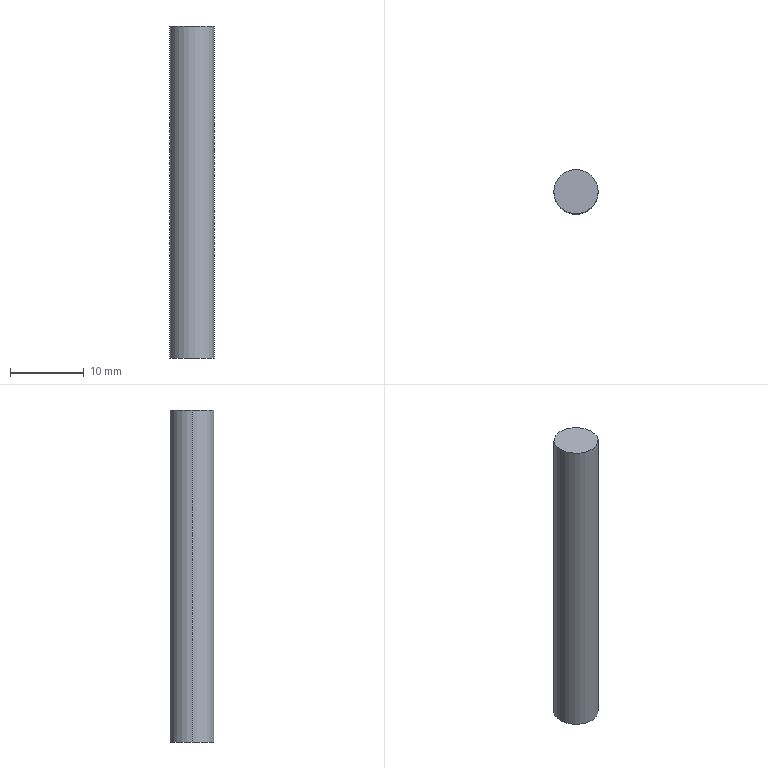Part | SolidWorks | features Extrusion 1 | 1 solid | 4 faces | box 6 x 6 x 45 mm | volume 1272 mm3 | cylinder 2 | plane 2 | commonest cylinder face diameters 6 x2
STEP:
#1=CARTESIAN_POINT('',(3.,0.,22.5));
#2=VERTEX_POINT('',#1);
#3=CARTESIAN_POINT('',(-3.,0.,22.5));
#4=VERTEX_POINT('',#3);
#5=CARTESIAN_POINT('',(0.,0.,22.5));
#6=DIRECTION('',(0.,0.,1.));
#7=DIRECTION('',(1.,0.,0.));
#8=AXIS2_PLACEMENT_3D('',#5,#6,#7);
#9=CIRCLE('',#8,3.);
#10=EDGE_CURVE('',#2,#4,#9,.T.);
#11=ORIENTED_EDGE('',*,*,#10,.F.);
#12=CARTESIAN_POINT('',(3.,0.,-22.5));
#13=VERTEX_POINT('',#12);
#14=CARTESIAN_POINT('',(3.,0.,22.5));
#15=DIRECTION('',(0.,0.,-1.));
#16=VECTOR('',#15,1000.);
#17=LINE('',#14,#16);
#18=EDGE_CURVE('',#2,#13,#17,.T.);
#19=ORIENTED_EDGE('',*,*,#18,.T.);
#20=CARTESIAN_POINT('',(-3.,0.,-22.5));
#21=VERTEX_POINT('',#20);
#22=CARTESIAN_POINT('',(0.,0.,-22.5));
#23=DIRECTION('',(0.,0.,1.));
#24=DIRECTION('',(1.,0.,0.));
#25=AXIS2_PLACEMENT_3D('',#22,#23,#24);
#26=CIRCLE('',#25,3.);
#27=EDGE_CURVE('',#13,#21,#26,.T.);
#28=ORIENTED_EDGE('',*,*,#27,.T.);
#29=CARTESIAN_POINT('',(-3.,0.,22.5));
#30=DIRECTION('',(0.,0.,-1.));
#31=VECTOR('',#30,1000.);
#32=LINE('',#29,#31);
#33=EDGE_CURVE('',#4,#21,#32,.T.);
#34=ORIENTED_EDGE('',*,*,#33,.F.);
#35=EDGE_LOOP('',(#11,#19,#28,#34));
#36=FACE_OUTER_BOUND('',#35,.T.);
#37=CARTESIAN_POINT('',(0.,0.,22.5));
#38=DIRECTION('',(0.,0.,-1.));
#39=DIRECTION('',(-1.,0.,0.));
#40=AXIS2_PLACEMENT_3D('',#37,#38,#39);
#41=CYLINDRICAL_SURFACE('',#40,3.);
#42=ADVANCED_FACE('',(#36),#41,.T.);
#43=ORIENTED_EDGE('',*,*,#18,.F.);
#44=CARTESIAN_POINT('',(0.,0.,22.5));
#45=DIRECTION('',(0.,0.,1.));
#46=DIRECTION('',(1.,0.,0.));
#47=AXIS2_PLACEMENT_3D('',#44,#45,#46);
#48=CIRCLE('',#47,3.);
#49=EDGE_CURVE('',#4,#2,#48,.T.);
#50=ORIENTED_EDGE('',*,*,#49,.F.);
#51=ORIENTED_EDGE('',*,*,#33,.T.);
#52=CARTESIAN_POINT('',(0.,0.,-22.5));
#53=DIRECTION('',(0.,0.,1.));
#54=DIRECTION('',(1.,0.,0.));
#55=AXIS2_PLACEMENT_3D('',#52,#53,#54);
#56=CIRCLE('',#55,3.);
#57=EDGE_CURVE('',#21,#13,#56,.T.);
#58=ORIENTED_EDGE('',*,*,#57,.T.);
#59=EDGE_LOOP('',(#43,#50,#51,#58));
#60=FACE_OUTER_BOUND('',#59,.T.);
#61=CARTESIAN_POINT('',(0.,0.,22.5));
#62=DIRECTION('',(0.,0.,-1.));
#63=DIRECTION('',(-1.,0.,0.));
#64=AXIS2_PLACEMENT_3D('',#61,#62,#63);
#65=CYLINDRICAL_SURFACE('',#64,3.);
#66=ADVANCED_FACE('',(#60),#65,.T.);
#67=ORIENTED_EDGE('',*,*,#49,.T.);
#68=ORIENTED_EDGE('',*,*,#10,.T.);
#69=EDGE_LOOP('',(#67,#68));
#70=FACE_OUTER_BOUND('',#69,.T.);
#71=CARTESIAN_POINT('',(0.,0.,22.5));
#72=DIRECTION('',(0.,0.,1.));
#73=DIRECTION('',(1.,0.,0.));
#74=AXIS2_PLACEMENT_3D('',#71,#72,#73);
#75=PLANE('',#74);
#76=ADVANCED_FACE('',(#70),#75,.T.);
#77=ORIENTED_EDGE('',*,*,#57,.F.);
#78=ORIENTED_EDGE('',*,*,#27,.F.);
#79=EDGE_LOOP('',(#77,#78));
#80=FACE_OUTER_BOUND('',#79,.T.);
#81=CARTESIAN_POINT('',(0.,0.,-22.5));
#82=DIRECTION('',(0.,0.,1.));
#83=DIRECTION('',(1.,0.,0.));
#84=AXIS2_PLACEMENT_3D('',#81,#82,#83);
#85=PLANE('',#84);
#86=ADVANCED_FACE('',(#80),#85,.F.);
#87=CLOSED_SHELL('',(#42,#66,#76,#86));
#88=MANIFOLD_SOLID_BREP('',#87);
#89=CARTESIAN_POINT('',(0.,0.,0.));
#90=DIRECTION('',(0.,0.,1.));
#91=DIRECTION('',(1.,0.,0.));
#92=AXIS2_PLACEMENT_3D('',#89,#90,#91);
#93=(LENGTH_UNIT()NAMED_UNIT(*)SI_UNIT(.MILLI.,.METRE.));
#94=UNCERTAINTY_MEASURE_WITH_UNIT(LENGTH_MEASURE(0.00001),#93,'','');
#95=(NAMED_UNIT(*)PLANE_ANGLE_UNIT()SI_UNIT($,.RADIAN.));
#96=(NAMED_UNIT(*)SI_UNIT($,.STERADIAN.)SOLID_ANGLE_UNIT());
#97=(GEOMETRIC_REPRESENTATION_CONTEXT(3)GLOBAL_UNCERTAINTY_ASSIGNED_CONTEXT((#94))GLOBAL_UNIT_ASSIGNED_CONTEXT((#93,#95,#96))REPRESENTATION_CONTEXT('',''));
#98=ADVANCED_BREP_SHAPE_REPRESENTATION('',(#88,#92),#97);